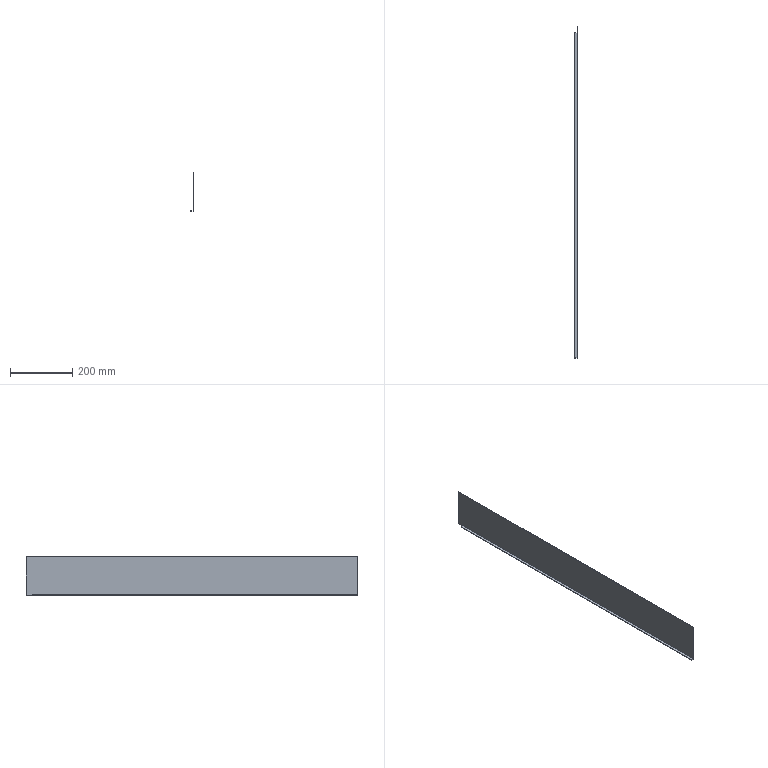Part | SolidWorks | 1 solid | 18 faces | box 10 x 1070 x 125 mm | volume 213423 mm3 | plane 16 | cylinder 2 | commonest cylinder face diameters 0.2 x1 3.2 x1
STEP:
#1=CARTESIAN_POINT('',(0.,514.75,-62.5));
#2=VERTEX_POINT('',#1);
#3=CARTESIAN_POINT('',(0.,535.,-62.5));
#4=VERTEX_POINT('',#3);
#5=CARTESIAN_POINT('',(0.,-535.,-62.5));
#6=DIRECTION('',(0.,1.,0.));
#7=VECTOR('',#6,1000.);
#8=LINE('',#5,#7);
#9=EDGE_CURVE('',#2,#4,#8,.T.);
#10=ORIENTED_EDGE('',*,*,#9,.F.);
#11=CARTESIAN_POINT('',(-1.5,514.75,-62.5));
#12=VERTEX_POINT('',#11);
#13=CARTESIAN_POINT('',(-1.5,514.75,-62.5));
#14=DIRECTION('',(1.,0.,0.));
#15=VECTOR('',#14,1000.);
#16=LINE('',#13,#15);
#17=EDGE_CURVE('',#12,#2,#16,.T.);
#18=ORIENTED_EDGE('',*,*,#17,.F.);
#19=CARTESIAN_POINT('',(-1.5,535.,-62.5));
#20=VERTEX_POINT('',#19);
#21=CARTESIAN_POINT('',(-1.5,-535.,-62.5));
#22=DIRECTION('',(0.,1.,0.));
#23=VECTOR('',#22,1000.);
#24=LINE('',#21,#23);
#25=EDGE_CURVE('',#12,#20,#24,.T.);
#26=ORIENTED_EDGE('',*,*,#25,.T.);
#27=CARTESIAN_POINT('',(-1.5,535.,-62.5));
#28=DIRECTION('',(1.,0.,0.));
#29=VECTOR('',#28,1000.);
#30=LINE('',#27,#29);
#31=EDGE_CURVE('',#20,#4,#30,.T.);
#32=ORIENTED_EDGE('',*,*,#31,.T.);
#33=EDGE_LOOP('',(#10,#18,#26,#32));
#34=FACE_OUTER_BOUND('',#33,.T.);
#35=CARTESIAN_POINT('',(-1.5,-535.,-62.5));
#36=DIRECTION('',(0.,0.,-1.));
#37=DIRECTION('',(-1.,0.,0.));
#38=AXIS2_PLACEMENT_3D('',#35,#36,#37);
#39=PLANE('',#38);
#40=ADVANCED_FACE('',(#34),#39,.T.);
#41=CARTESIAN_POINT('',(-1.5,-535.,62.5));
#42=VERTEX_POINT('',#41);
#43=CARTESIAN_POINT('',(-1.5,-535.,-60.9));
#44=VERTEX_POINT('',#43);
#45=CARTESIAN_POINT('',(-1.5,-535.,-62.5));
#46=DIRECTION('',(0.,0.,-1.));
#47=VECTOR('',#46,1000.);
#48=LINE('',#45,#47);
#49=EDGE_CURVE('',#42,#44,#48,.T.);
#50=ORIENTED_EDGE('',*,*,#49,.T.);
#51=CARTESIAN_POINT('',(0.,-535.,-60.9));
#52=VERTEX_POINT('',#51);
#53=CARTESIAN_POINT('',(-1.5,-535.,-60.9));
#54=DIRECTION('',(1.,0.,0.));
#55=VECTOR('',#54,1000.);
#56=LINE('',#53,#55);
#57=EDGE_CURVE('',#44,#52,#56,.T.);
#58=ORIENTED_EDGE('',*,*,#57,.T.);
#59=CARTESIAN_POINT('',(0.,-535.,62.5));
#60=VERTEX_POINT('',#59);
#61=CARTESIAN_POINT('',(0.,-535.,-62.5));
#62=DIRECTION('',(0.,0.,-1.));
#63=VECTOR('',#62,1000.);
#64=LINE('',#61,#63);
#65=EDGE_CURVE('',#60,#52,#64,.T.);
#66=ORIENTED_EDGE('',*,*,#65,.F.);
#67=CARTESIAN_POINT('',(-1.5,-535.,62.5));
#68=DIRECTION('',(1.,0.,0.));
#69=VECTOR('',#68,1000.);
#70=LINE('',#67,#69);
#71=EDGE_CURVE('',#42,#60,#70,.T.);
#72=ORIENTED_EDGE('',*,*,#71,.F.);
#73=EDGE_LOOP('',(#50,#58,#66,#72));
#74=FACE_OUTER_BOUND('',#73,.T.);
#75=CARTESIAN_POINT('',(-1.5,-535.,-62.5));
#76=DIRECTION('',(0.,-1.,0.));
#77=DIRECTION('',(0.,0.,-1.));
#78=AXIS2_PLACEMENT_3D('',#75,#76,#77);
#79=PLANE('',#78);
#80=ADVANCED_FACE('',(#74),#79,.T.);
#81=CARTESIAN_POINT('',(-1.5,514.,-60.9));
#82=VERTEX_POINT('',#81);
#83=CARTESIAN_POINT('',(-1.5,-535.,-60.9));
#84=DIRECTION('',(0.,1.,0.));
#85=VECTOR('',#84,1000.);
#86=LINE('',#83,#85);
#87=EDGE_CURVE('',#44,#82,#86,.T.);
#88=ORIENTED_EDGE('',*,*,#87,.F.);
#89=ORIENTED_EDGE('',*,*,#49,.F.);
#90=CARTESIAN_POINT('',(-1.5,535.,62.5));
#91=VERTEX_POINT('',#90);
#92=CARTESIAN_POINT('',(-1.5,-535.,62.5));
#93=DIRECTION('',(0.,-1.,0.));
#94=VECTOR('',#93,1000.);
#95=LINE('',#92,#94);
#96=EDGE_CURVE('',#91,#42,#95,.T.);
#97=ORIENTED_EDGE('',*,*,#96,.F.);
#98=CARTESIAN_POINT('',(-1.5,535.,-62.5));
#99=DIRECTION('',(0.,0.,1.));
#100=VECTOR('',#99,1000.);
#101=LINE('',#98,#100);
#102=EDGE_CURVE('',#20,#91,#101,.T.);
#103=ORIENTED_EDGE('',*,*,#102,.F.);
#104=ORIENTED_EDGE('',*,*,#25,.F.);
#105=CARTESIAN_POINT('',(-1.5,514.75,-60.15));
#106=VERTEX_POINT('',#105);
#107=CARTESIAN_POINT('',(-1.5,514.75,-60.15));
#108=DIRECTION('',(0.,0.,-1.));
#109=VECTOR('',#108,1000.);
#110=LINE('',#107,#109);
#111=EDGE_CURVE('',#106,#12,#110,.T.);
#112=ORIENTED_EDGE('',*,*,#111,.F.);
#113=CARTESIAN_POINT('',(-1.5,514.,-60.15));
#114=VERTEX_POINT('',#113);
#115=CARTESIAN_POINT('',(-1.5,514.,-60.15));
#116=DIRECTION('',(0.,1.,0.));
#117=VECTOR('',#116,1000.);
#118=LINE('',#115,#117);
#119=EDGE_CURVE('',#114,#106,#118,.T.);
#120=ORIENTED_EDGE('',*,*,#119,.F.);
#121=CARTESIAN_POINT('',(-1.5,514.,-60.9));
#122=DIRECTION('',(0.,0.,1.));
#123=VECTOR('',#122,1000.);
#124=LINE('',#121,#123);
#125=EDGE_CURVE('',#82,#114,#124,.T.);
#126=ORIENTED_EDGE('',*,*,#125,.F.);
#127=EDGE_LOOP('',(#88,#89,#97,#103,#104,#112,#120,#126));
#128=FACE_OUTER_BOUND('',#127,.T.);
#129=CARTESIAN_POINT('',(-1.5,0.,0.));
#130=DIRECTION('',(1.,0.,0.));
#131=DIRECTION('',(0.,0.,-1.));
#132=AXIS2_PLACEMENT_3D('',#129,#130,#131);
#133=PLANE('',#132);
#134=ADVANCED_FACE('',(#128),#133,.F.);
#135=ORIENTED_EDGE('',*,*,#65,.T.);
#136=CARTESIAN_POINT('',(0.,514.,-60.9));
#137=VERTEX_POINT('',#136);
#138=CARTESIAN_POINT('',(0.,-535.,-60.9));
#139=DIRECTION('',(0.,1.,0.));
#140=VECTOR('',#139,1000.);
#141=LINE('',#138,#140);
#142=EDGE_CURVE('',#52,#137,#141,.T.);
#143=ORIENTED_EDGE('',*,*,#142,.T.);
#144=CARTESIAN_POINT('',(0.,514.,-60.15));
#145=VERTEX_POINT('',#144);
#146=CARTESIAN_POINT('',(0.,514.,0.));
#147=DIRECTION('',(0.,0.,1.));
#148=VECTOR('',#147,1000.);
#149=LINE('',#146,#148);
#150=EDGE_CURVE('',#137,#145,#149,.T.);
#151=ORIENTED_EDGE('',*,*,#150,.T.);
#152=CARTESIAN_POINT('',(0.,514.75,-60.15));
#153=VERTEX_POINT('',#152);
#154=CARTESIAN_POINT('',(0.,0.,-60.15));
#155=DIRECTION('',(0.,1.,0.));
#156=VECTOR('',#155,1000.);
#157=LINE('',#154,#156);
#158=EDGE_CURVE('',#145,#153,#157,.T.);
#159=ORIENTED_EDGE('',*,*,#158,.T.);
#160=CARTESIAN_POINT('',(0.,514.75,0.));
#161=DIRECTION('',(0.,0.,-1.));
#162=VECTOR('',#161,1000.);
#163=LINE('',#160,#162);
#164=EDGE_CURVE('',#153,#2,#163,.T.);
#165=ORIENTED_EDGE('',*,*,#164,.T.);
#166=ORIENTED_EDGE('',*,*,#9,.T.);
#167=CARTESIAN_POINT('',(0.,535.,62.5));
#168=VERTEX_POINT('',#167);
#169=CARTESIAN_POINT('',(0.,535.,-62.5));
#170=DIRECTION('',(0.,0.,1.));
#171=VECTOR('',#170,1000.);
#172=LINE('',#169,#171);
#173=EDGE_CURVE('',#4,#168,#172,.T.);
#174=ORIENTED_EDGE('',*,*,#173,.T.);
#175=CARTESIAN_POINT('',(0.,-535.,62.5));
#176=DIRECTION('',(0.,-1.,0.));
#177=VECTOR('',#176,1000.);
#178=LINE('',#175,#177);
#179=EDGE_CURVE('',#168,#60,#178,.T.);
#180=ORIENTED_EDGE('',*,*,#179,.T.);
#181=EDGE_LOOP('',(#135,#143,#151,#159,#165,#166,#174,#180));
#182=FACE_OUTER_BOUND('',#181,.T.);
#183=CARTESIAN_POINT('',(0.,0.,0.));
#184=DIRECTION('',(1.,0.,0.));
#185=DIRECTION('',(0.,0.,-1.));
#186=AXIS2_PLACEMENT_3D('',#183,#184,#185);
#187=PLANE('',#186);
#188=ADVANCED_FACE('',(#182),#187,.T.);
#189=ORIENTED_EDGE('',*,*,#179,.F.);
#190=CARTESIAN_POINT('',(-1.5,535.,62.5));
#191=DIRECTION('',(1.,0.,0.));
#192=VECTOR('',#191,1000.);
#193=LINE('',#190,#192);
#194=EDGE_CURVE('',#91,#168,#193,.T.);
#195=ORIENTED_EDGE('',*,*,#194,.F.);
#196=ORIENTED_EDGE('',*,*,#96,.T.);
#197=ORIENTED_EDGE('',*,*,#71,.T.);
#198=EDGE_LOOP('',(#189,#195,#196,#197));
#199=FACE_OUTER_BOUND('',#198,.T.);
#200=CARTESIAN_POINT('',(-1.5,-535.,62.5));
#201=DIRECTION('',(0.,0.,1.));
#202=DIRECTION('',(0.,-1.,0.));
#203=AXIS2_PLACEMENT_3D('',#200,#201,#202);
#204=PLANE('',#203);
#205=ADVANCED_FACE('',(#199),#204,.T.);
#206=ORIENTED_EDGE('',*,*,#173,.F.);
#207=ORIENTED_EDGE('',*,*,#31,.F.);
#208=ORIENTED_EDGE('',*,*,#102,.T.);
#209=ORIENTED_EDGE('',*,*,#194,.T.);
#210=EDGE_LOOP('',(#206,#207,#208,#209));
#211=FACE_OUTER_BOUND('',#210,.T.);
#212=CARTESIAN_POINT('',(-1.5,535.,-62.5));
#213=DIRECTION('',(0.,1.,0.));
#214=DIRECTION('',(0.,0.,1.));
#215=AXIS2_PLACEMENT_3D('',#212,#213,#214);
#216=PLANE('',#215);
#217=ADVANCED_FACE('',(#211),#216,.T.);
#218=ORIENTED_EDGE('',*,*,#150,.F.);
#219=CARTESIAN_POINT('',(-1.5,514.,-60.9));
#220=DIRECTION('',(1.,0.,0.));
#221=VECTOR('',#220,1000.);
#222=LINE('',#219,#221);
#223=EDGE_CURVE('',#82,#137,#222,.T.);
#224=ORIENTED_EDGE('',*,*,#223,.F.);
#225=ORIENTED_EDGE('',*,*,#125,.T.);
#226=CARTESIAN_POINT('',(-1.5,514.,-60.15));
#227=DIRECTION('',(1.,0.,0.));
#228=VECTOR('',#227,1000.);
#229=LINE('',#226,#228);
#230=EDGE_CURVE('',#114,#145,#229,.T.);
#231=ORIENTED_EDGE('',*,*,#230,.T.);
#232=EDGE_LOOP('',(#218,#224,#225,#231));
#233=FACE_OUTER_BOUND('',#232,.T.);
#234=CARTESIAN_POINT('',(-1.5,514.,-60.9));
#235=DIRECTION('',(0.,1.,0.));
#236=DIRECTION('',(0.,0.,1.));
#237=AXIS2_PLACEMENT_3D('',#234,#235,#236);
#238=PLANE('',#237);
#239=ADVANCED_FACE('',(#233),#238,.T.);
#240=ORIENTED_EDGE('',*,*,#158,.F.);
#241=ORIENTED_EDGE('',*,*,#230,.F.);
#242=ORIENTED_EDGE('',*,*,#119,.T.);
#243=CARTESIAN_POINT('',(-1.5,514.75,-60.15));
#244=DIRECTION('',(1.,0.,0.));
#245=VECTOR('',#244,1000.);
#246=LINE('',#243,#245);
#247=EDGE_CURVE('',#106,#153,#246,.T.);
#248=ORIENTED_EDGE('',*,*,#247,.T.);
#249=EDGE_LOOP('',(#240,#241,#242,#248));
#250=FACE_OUTER_BOUND('',#249,.T.);
#251=CARTESIAN_POINT('',(-1.5,514.,-60.15));
#252=DIRECTION('',(0.,0.,-1.));
#253=DIRECTION('',(-1.,0.,0.));
#254=AXIS2_PLACEMENT_3D('',#251,#252,#253);
#255=PLANE('',#254);
#256=ADVANCED_FACE('',(#250),#255,.T.);
#257=ORIENTED_EDGE('',*,*,#164,.F.);
#258=ORIENTED_EDGE('',*,*,#247,.F.);
#259=ORIENTED_EDGE('',*,*,#111,.T.);
#260=ORIENTED_EDGE('',*,*,#17,.T.);
#261=EDGE_LOOP('',(#257,#258,#259,#260));
#262=FACE_OUTER_BOUND('',#261,.T.);
#263=CARTESIAN_POINT('',(-1.5,514.75,-60.15));
#264=DIRECTION('',(0.,-1.,0.));
#265=DIRECTION('',(0.,0.,-1.));
#266=AXIS2_PLACEMENT_3D('',#263,#264,#265);
#267=PLANE('',#266);
#268=ADVANCED_FACE('',(#262),#267,.T.);
#269=CARTESIAN_POINT('',(-1.6,514.,-61.));
#270=VERTEX_POINT('',#269);
#271=CARTESIAN_POINT('',(-1.6,514.,-62.5));
#272=VERTEX_POINT('',#271);
#273=CARTESIAN_POINT('',(-1.6,514.,-62.5));
#274=DIRECTION('',(0.,0.,-1.));
#275=VECTOR('',#274,1000.);
#276=LINE('',#273,#275);
#277=EDGE_CURVE('',#270,#272,#276,.T.);
#278=ORIENTED_EDGE('',*,*,#277,.F.);
#279=CARTESIAN_POINT('',(-1.6,514.,-60.9));
#280=DIRECTION('',(0.,1.,0.));
#281=DIRECTION('',(0.,0.,-1.));
#282=AXIS2_PLACEMENT_3D('',#279,#280,#281);
#283=CIRCLE('',#282,0.1);
#284=EDGE_CURVE('',#82,#270,#283,.T.);
#285=ORIENTED_EDGE('',*,*,#284,.F.);
#286=ORIENTED_EDGE('',*,*,#223,.T.);
#287=CARTESIAN_POINT('',(-1.6,514.,-60.9));
#288=DIRECTION('',(0.,1.,0.));
#289=DIRECTION('',(0.,0.,-1.));
#290=AXIS2_PLACEMENT_3D('',#287,#288,#289);
#291=CIRCLE('',#290,1.6);
#292=EDGE_CURVE('',#137,#272,#291,.T.);
#293=ORIENTED_EDGE('',*,*,#292,.T.);
#294=EDGE_LOOP('',(#278,#285,#286,#293));
#295=FACE_OUTER_BOUND('',#294,.T.);
#296=CARTESIAN_POINT('',(-1.6,514.,-60.9));
#297=DIRECTION('',(0.,1.,0.));
#298=DIRECTION('',(0.,0.,1.));
#299=AXIS2_PLACEMENT_3D('',#296,#297,#298);
#300=PLANE('',#299);
#301=ADVANCED_FACE('',(#295),#300,.T.);
#302=CARTESIAN_POINT('',(-1.6,-535.,-61.));
#303=VERTEX_POINT('',#302);
#304=CARTESIAN_POINT('',(-1.6,-535.,-60.9));
#305=DIRECTION('',(0.,-1.,0.));
#306=DIRECTION('',(0.,0.,-1.));
#307=AXIS2_PLACEMENT_3D('',#304,#305,#306);
#308=CIRCLE('',#307,0.1);
#309=EDGE_CURVE('',#303,#44,#308,.T.);
#310=ORIENTED_EDGE('',*,*,#309,.F.);
#311=CARTESIAN_POINT('',(-1.6,-535.,-62.5));
#312=VERTEX_POINT('',#311);
#313=CARTESIAN_POINT('',(-1.6,-535.,-61.));
#314=DIRECTION('',(0.,0.,-1.));
#315=VECTOR('',#314,1000.);
#316=LINE('',#313,#315);
#317=EDGE_CURVE('',#303,#312,#316,.T.);
#318=ORIENTED_EDGE('',*,*,#317,.T.);
#319=CARTESIAN_POINT('',(-1.6,-535.,-60.9));
#320=DIRECTION('',(0.,-1.,0.));
#321=DIRECTION('',(0.,0.,-1.));
#322=AXIS2_PLACEMENT_3D('',#319,#320,#321);
#323=CIRCLE('',#322,1.6);
#324=EDGE_CURVE('',#312,#52,#323,.T.);
#325=ORIENTED_EDGE('',*,*,#324,.T.);
#326=ORIENTED_EDGE('',*,*,#57,.F.);
#327=EDGE_LOOP('',(#310,#318,#325,#326));
#328=FACE_OUTER_BOUND('',#327,.T.);
#329=CARTESIAN_POINT('',(-1.6,-535.,-60.9));
#330=DIRECTION('',(0.,1.,0.));
#331=DIRECTION('',(0.,0.,1.));
#332=AXIS2_PLACEMENT_3D('',#329,#330,#331);
#333=PLANE('',#332);
#334=ADVANCED_FACE('',(#328),#333,.F.);
#335=ORIENTED_EDGE('',*,*,#142,.F.);
#336=ORIENTED_EDGE('',*,*,#324,.F.);
#337=CARTESIAN_POINT('',(-1.6,514.,-62.5));
#338=DIRECTION('',(0.,1.,0.));
#339=VECTOR('',#338,1000.);
#340=LINE('',#337,#339);
#341=EDGE_CURVE('',#312,#272,#340,.T.);
#342=ORIENTED_EDGE('',*,*,#341,.T.);
#343=ORIENTED_EDGE('',*,*,#292,.F.);
#344=EDGE_LOOP('',(#335,#336,#342,#343));
#345=FACE_OUTER_BOUND('',#344,.T.);
#346=CARTESIAN_POINT('',(-1.6,-535.,-60.9));
#347=DIRECTION('',(0.,-1.,0.));
#348=DIRECTION('',(0.,0.,-1.));
#349=AXIS2_PLACEMENT_3D('',#346,#347,#348);
#350=CYLINDRICAL_SURFACE('',#349,1.6);
#351=ADVANCED_FACE('',(#345),#350,.T.);
#352=ORIENTED_EDGE('',*,*,#87,.T.);
#353=ORIENTED_EDGE('',*,*,#284,.T.);
#354=CARTESIAN_POINT('',(-1.6,514.,-61.));
#355=DIRECTION('',(0.,-1.,0.));
#356=VECTOR('',#355,1000.);
#357=LINE('',#354,#356);
#358=EDGE_CURVE('',#270,#303,#357,.T.);
#359=ORIENTED_EDGE('',*,*,#358,.T.);
#360=ORIENTED_EDGE('',*,*,#309,.T.);
#361=EDGE_LOOP('',(#352,#353,#359,#360));
#362=FACE_OUTER_BOUND('',#361,.T.);
#363=CARTESIAN_POINT('',(-1.6,-535.,-60.9));
#364=DIRECTION('',(0.,-1.,0.));
#365=DIRECTION('',(0.,0.,-1.));
#366=AXIS2_PLACEMENT_3D('',#363,#364,#365);
#367=CYLINDRICAL_SURFACE('',#366,0.1);
#368=ADVANCED_FACE('',(#362),#367,.F.);
#369=ORIENTED_EDGE('',*,*,#317,.F.);
#370=CARTESIAN_POINT('',(-10.,-535.,-61.));
#371=VERTEX_POINT('',#370);
#372=CARTESIAN_POINT('',(-10.,-535.,-61.));
#373=DIRECTION('',(-1.,0.,0.));
#374=VECTOR('',#373,1000.);
#375=LINE('',#372,#374);
#376=EDGE_CURVE('',#303,#371,#375,.T.);
#377=ORIENTED_EDGE('',*,*,#376,.T.);
#378=CARTESIAN_POINT('',(-10.,-535.,-62.5));
#379=VERTEX_POINT('',#378);
#380=CARTESIAN_POINT('',(-10.,-535.,-62.5));
#381=DIRECTION('',(0.,0.,1.));
#382=VECTOR('',#381,1000.);
#383=LINE('',#380,#382);
#384=EDGE_CURVE('',#379,#371,#383,.T.);
#385=ORIENTED_EDGE('',*,*,#384,.F.);
#386=CARTESIAN_POINT('',(0.,-535.,-62.5));
#387=DIRECTION('',(-1.,0.,0.));
#388=VECTOR('',#387,1000.);
#389=LINE('',#386,#388);
#390=EDGE_CURVE('',#312,#379,#389,.T.);
#391=ORIENTED_EDGE('',*,*,#390,.F.);
#392=EDGE_LOOP('',(#369,#377,#385,#391));
#393=FACE_OUTER_BOUND('',#392,.T.);
#394=CARTESIAN_POINT('',(-10.,-535.,-62.5));
#395=DIRECTION('',(0.,1.,0.));
#396=DIRECTION('',(0.,0.,1.));
#397=AXIS2_PLACEMENT_3D('',#394,#395,#396);
#398=PLANE('',#397);
#399=ADVANCED_FACE('',(#393),#398,.F.);
#400=ORIENTED_EDGE('',*,*,#277,.T.);
#401=CARTESIAN_POINT('',(-10.,514.,-62.5));
#402=VERTEX_POINT('',#401);
#403=CARTESIAN_POINT('',(0.,514.,-62.5));
#404=DIRECTION('',(1.,0.,0.));
#405=VECTOR('',#404,1000.);
#406=LINE('',#403,#405);
#407=EDGE_CURVE('',#402,#272,#406,.T.);
#408=ORIENTED_EDGE('',*,*,#407,.F.);
#409=CARTESIAN_POINT('',(-10.,514.,-61.));
#410=VERTEX_POINT('',#409);
#411=CARTESIAN_POINT('',(-10.,514.,-62.5));
#412=DIRECTION('',(0.,0.,1.));
#413=VECTOR('',#412,1000.);
#414=LINE('',#411,#413);
#415=EDGE_CURVE('',#402,#410,#414,.T.);
#416=ORIENTED_EDGE('',*,*,#415,.T.);
#417=CARTESIAN_POINT('',(-1.5,514.,-61.));
#418=DIRECTION('',(1.,0.,0.));
#419=VECTOR('',#418,1000.);
#420=LINE('',#417,#419);
#421=EDGE_CURVE('',#410,#270,#420,.T.);
#422=ORIENTED_EDGE('',*,*,#421,.T.);
#423=EDGE_LOOP('',(#400,#408,#416,#422));
#424=FACE_OUTER_BOUND('',#423,.T.);
#425=CARTESIAN_POINT('',(-1.5,514.,-62.5));
#426=DIRECTION('',(0.,-1.,0.));
#427=DIRECTION('',(1.,0.,0.));
#428=AXIS2_PLACEMENT_3D('',#425,#426,#427);
#429=PLANE('',#428);
#430=ADVANCED_FACE('',(#424),#429,.F.);
#431=ORIENTED_EDGE('',*,*,#341,.F.);
#432=ORIENTED_EDGE('',*,*,#390,.T.);
#433=CARTESIAN_POINT('',(-10.,0.,-62.5));
#434=DIRECTION('',(0.,1.,0.));
#435=VECTOR('',#434,1000.);
#436=LINE('',#433,#435);
#437=EDGE_CURVE('',#379,#402,#436,.T.);
#438=ORIENTED_EDGE('',*,*,#437,.T.);
#439=ORIENTED_EDGE('',*,*,#407,.T.);
#440=EDGE_LOOP('',(#431,#432,#438,#439));
#441=FACE_OUTER_BOUND('',#440,.T.);
#442=CARTESIAN_POINT('',(0.,0.,-62.5));
#443=DIRECTION('',(0.,0.,1.));
#444=DIRECTION('',(1.,0.,0.));
#445=AXIS2_PLACEMENT_3D('',#442,#443,#444);
#446=PLANE('',#445);
#447=ADVANCED_FACE('',(#441),#446,.F.);
#448=ORIENTED_EDGE('',*,*,#376,.F.);
#449=ORIENTED_EDGE('',*,*,#358,.F.);
#450=ORIENTED_EDGE('',*,*,#421,.F.);
#451=CARTESIAN_POINT('',(-10.,514.,-61.));
#452=DIRECTION('',(0.,1.,0.));
#453=VECTOR('',#452,1000.);
#454=LINE('',#451,#453);
#455=EDGE_CURVE('',#371,#410,#454,.T.);
#456=ORIENTED_EDGE('',*,*,#455,.F.);
#457=EDGE_LOOP('',(#448,#449,#450,#456));
#458=FACE_OUTER_BOUND('',#457,.T.);
#459=CARTESIAN_POINT('',(0.,0.,-61.));
#460=DIRECTION('',(0.,0.,1.));
#461=DIRECTION('',(1.,0.,0.));
#462=AXIS2_PLACEMENT_3D('',#459,#460,#461);
#463=PLANE('',#462);
#464=ADVANCED_FACE('',(#458),#463,.T.);
#465=ORIENTED_EDGE('',*,*,#455,.T.);
#466=ORIENTED_EDGE('',*,*,#415,.F.);
#467=ORIENTED_EDGE('',*,*,#437,.F.);
#468=ORIENTED_EDGE('',*,*,#384,.T.);
#469=EDGE_LOOP('',(#465,#466,#467,#468));
#470=FACE_OUTER_BOUND('',#469,.T.);
#471=CARTESIAN_POINT('',(-10.,514.,-62.5));
#472=DIRECTION('',(1.,0.,0.));
#473=DIRECTION('',(0.,0.,-1.));
#474=AXIS2_PLACEMENT_3D('',#471,#472,#473);
#475=PLANE('',#474);
#476=ADVANCED_FACE('',(#470),#475,.F.);
#477=CLOSED_SHELL('',(#40,#80,#134,#188,#205,#217,#239,#256,#268,#301,#334,#351,#368,#399,#430,#447,#464,#476));
#478=MANIFOLD_SOLID_BREP('',#477);
#479=CARTESIAN_POINT('',(0.,0.,0.));
#480=DIRECTION('',(0.,0.,1.));
#481=DIRECTION('',(1.,0.,0.));
#482=AXIS2_PLACEMENT_3D('',#479,#480,#481);
#483=(LENGTH_UNIT()NAMED_UNIT(*)SI_UNIT(.MILLI.,.METRE.));
#484=UNCERTAINTY_MEASURE_WITH_UNIT(LENGTH_MEASURE(0.00001),#483,'','');
#485=(NAMED_UNIT(*)PLANE_ANGLE_UNIT()SI_UNIT($,.RADIAN.));
#486=(NAMED_UNIT(*)SI_UNIT($,.STERADIAN.)SOLID_ANGLE_UNIT());
#487=(GEOMETRIC_REPRESENTATION_CONTEXT(3)GLOBAL_UNCERTAINTY_ASSIGNED_CONTEXT((#484))GLOBAL_UNIT_ASSIGNED_CONTEXT((#483,#485,#486))REPRESENTATION_CONTEXT('',''));
#488=ADVANCED_BREP_SHAPE_REPRESENTATION('',(#478,#482),#487);